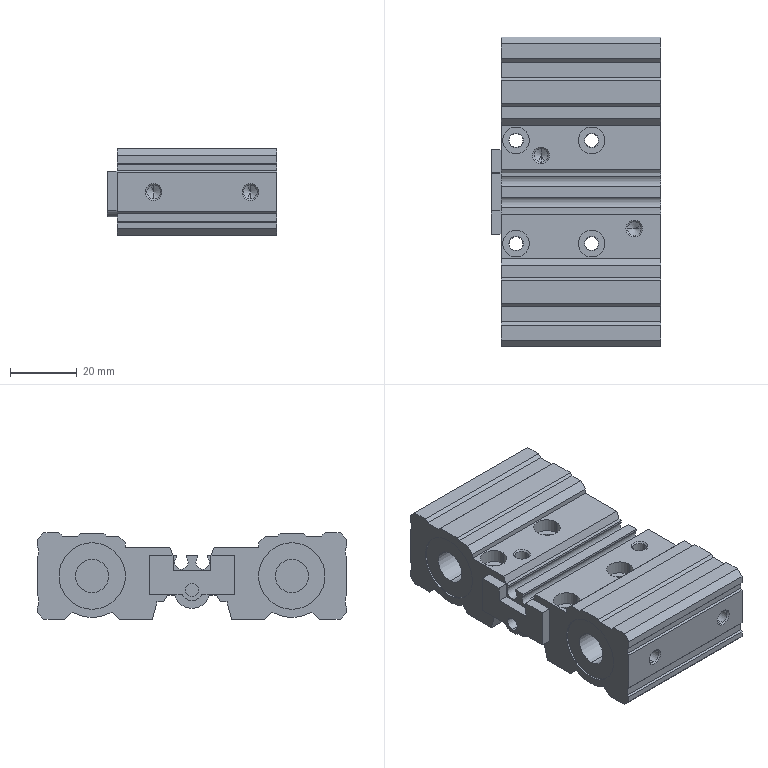Part | STEP file | 2-1 | 1 solid | 231 faces | box 51 x 93 x 26 mm | volume 74170 mm3 | plane 100 | cylinder 75 | cone 56 | commonest cylinder face diameters 4.134 x32 20 x12 4.3 x8 8 x8 10 x4 4 x2